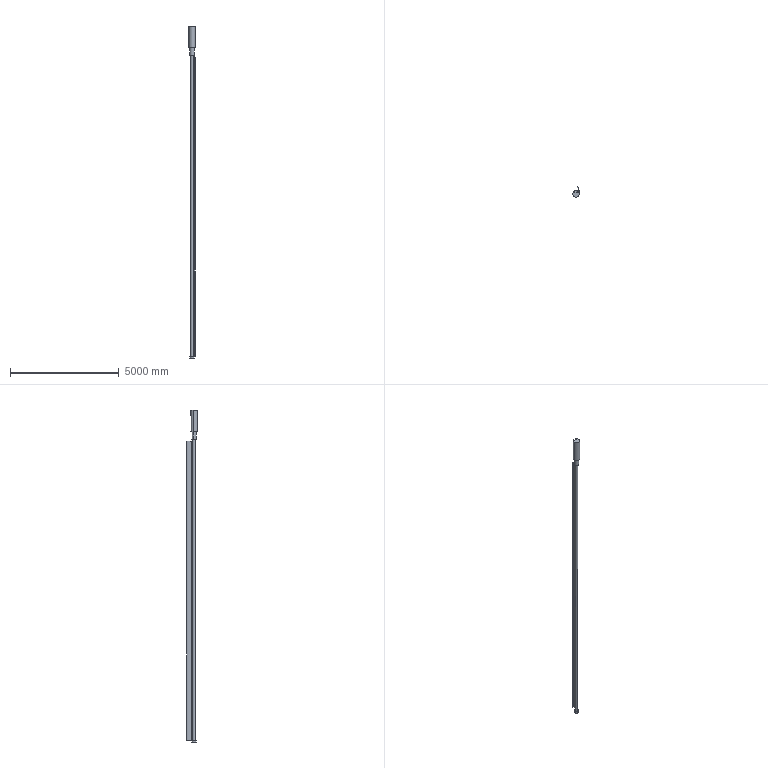Part | SolidWorks | features ICE 6, Extrusion 1 | 1 solid | 28 faces | box 300 x 474.612 x 15244 mm | volume 386924782 mm3 | plane 19 | cylinder 9 | commonest cylinder face diameters 200 x4 100 x2 300 x2 117.35 x1
STEP:
#1=CARTESIAN_POINT('',(50.,141.421,1160.));
#2=VERTEX_POINT('',#1);
#3=CARTESIAN_POINT('',(0.,150.,1110.));
#4=VERTEX_POINT('',#3);
#5=CARTESIAN_POINT('',(50.,141.421,1160.));
#6=CARTESIAN_POINT('',(50.,141.421,1156.669));
#7=CARTESIAN_POINT('',(49.671,141.539,1153.4));
#8=CARTESIAN_POINT('',(48.706,141.873,1148.582));
#9=CARTESIAN_POINT('',(48.306,142.01,1146.99));
#10=CARTESIAN_POINT('',(47.584,142.253,1144.624));
#11=CARTESIAN_POINT('',(47.323,142.34,1143.837));
#12=CARTESIAN_POINT('',(46.764,142.524,1142.286));
#13=CARTESIAN_POINT('',(46.467,142.622,1141.52));
#14=CARTESIAN_POINT('',(44.893,143.131,1137.743));
#15=CARTESIAN_POINT('',(43.355,143.61,1134.88));
#16=CARTESIAN_POINT('',(41.086,144.264,1131.494));
#17=CARTESIAN_POINT('',(40.615,144.398,1130.827));
#18=CARTESIAN_POINT('',(39.637,144.669,1129.511));
#19=CARTESIAN_POINT('',(39.132,144.807,1128.865));
#20=CARTESIAN_POINT('',(37.577,145.221,1126.975));
#21=CARTESIAN_POINT('',(36.486,145.5,1125.774));
#22=CARTESIAN_POINT('',(33.051,146.332,1122.342));
#23=CARTESIAN_POINT('',(30.547,146.883,1120.28));
#24=CARTESIAN_POINT('',(25.084,147.914,1116.623));
#25=CARTESIAN_POINT('',(22.213,148.377,1115.087));
#26=CARTESIAN_POINT('',(17.703,148.959,1113.211));
#27=CARTESIAN_POINT('',(16.166,149.135,1112.657));
#28=CARTESIAN_POINT('',(13.807,149.365,1111.937));
#29=CARTESIAN_POINT('',(13.012,149.437,1111.716));
#30=CARTESIAN_POINT('',(11.403,149.568,1111.311));
#31=CARTESIAN_POINT('',(10.595,149.628,1111.129));
#32=CARTESIAN_POINT('',(6.552,149.892,1110.322));
#33=CARTESIAN_POINT('',(3.29,150.,1110.));
#34=CARTESIAN_POINT('',(0.,150.,1110.));
#35=B_SPLINE_CURVE_WITH_KNOTS('',3,(#5,#6,#7,#8,#9,#10,#11,#12,#13,#14,#15,#16,#17,#18,#19,#20,#21,#22,#23,#24,#25,#26,#27,#28,#29,#30,#31,#32,#33,#34),.UNSPECIFIED.,.F.,.F.,(4,2,2,2,2,2,2,2,2,2,2,2,2,2,4),(0.,0.009844,0.01477,0.01723,0.01969,0.02953,0.03199,0.03445,0.03937,0.04922,0.05906,0.06398,0.06645,0.06891,0.07875),.UNSPECIFIED.);
#36=EDGE_CURVE('',#2,#4,#35,.T.);
#37=ORIENTED_EDGE('',*,*,#36,.T.);
#38=CARTESIAN_POINT('',(0.,75.,1110.));
#39=VERTEX_POINT('',#38);
#40=CARTESIAN_POINT('',(0.,326.,1110.));
#41=DIRECTION('',(0.,-1.,0.));
#42=VECTOR('',#41,1000.);
#43=LINE('',#40,#42);
#44=EDGE_CURVE('',#4,#39,#43,.T.);
#45=ORIENTED_EDGE('',*,*,#44,.T.);
#46=CARTESIAN_POINT('',(50.,75.,1160.));
#47=VERTEX_POINT('',#46);
#48=CARTESIAN_POINT('',(0.,75.,1160.));
#49=DIRECTION('',(0.,1.,0.));
#50=DIRECTION('',(0.,0.,1.));
#51=AXIS2_PLACEMENT_3D('',#48,#49,#50);
#52=CIRCLE('',#51,50.);
#53=EDGE_CURVE('',#47,#39,#52,.T.);
#54=ORIENTED_EDGE('',*,*,#53,.F.);
#55=CARTESIAN_POINT('',(50.,326.,1160.));
#56=DIRECTION('',(0.,-1.,0.));
#57=VECTOR('',#56,1000.);
#58=LINE('',#55,#57);
#59=EDGE_CURVE('',#2,#47,#58,.T.);
#60=ORIENTED_EDGE('',*,*,#59,.F.);
#61=EDGE_LOOP('',(#37,#45,#54,#60));
#62=FACE_OUTER_BOUND('',#61,.T.);
#63=CARTESIAN_POINT('',(0.,326.,1160.));
#64=DIRECTION('',(0.,-1.,0.));
#65=DIRECTION('',(0.,0.,-1.));
#66=AXIS2_PLACEMENT_3D('',#63,#64,#65);
#67=CYLINDRICAL_SURFACE('',#66,50.);
#68=ADVANCED_FACE('',(#62),#67,.F.);
#69=CARTESIAN_POINT('',(-100.,0.,-13904.));
#70=VERTEX_POINT('',#69);
#71=CARTESIAN_POINT('',(100.,0.,-13904.));
#72=VERTEX_POINT('',#71);
#73=CARTESIAN_POINT('',(0.,0.,-13904.));
#74=DIRECTION('',(0.,0.,-1.));
#75=DIRECTION('',(-1.,0.,0.));
#76=AXIS2_PLACEMENT_3D('',#73,#74,#75);
#77=CIRCLE('',#76,100.);
#78=EDGE_CURVE('',#70,#72,#77,.T.);
#79=ORIENTED_EDGE('',*,*,#78,.F.);
#80=CARTESIAN_POINT('',(-100.,0.,-13824.));
#81=VERTEX_POINT('',#80);
#82=CARTESIAN_POINT('',(-100.,0.,-13904.));
#83=DIRECTION('',(0.,0.,1.));
#84=VECTOR('',#83,1000.);
#85=LINE('',#82,#84);
#86=EDGE_CURVE('',#70,#81,#85,.T.);
#87=ORIENTED_EDGE('',*,*,#86,.T.);
#88=CARTESIAN_POINT('',(61.826,78.598,-13824.));
#89=VERTEX_POINT('',#88);
#90=CARTESIAN_POINT('',(0.,0.,-13824.));
#91=DIRECTION('',(0.,0.,-1.));
#92=DIRECTION('',(-1.,0.,0.));
#93=AXIS2_PLACEMENT_3D('',#90,#91,#92);
#94=CIRCLE('',#93,100.);
#95=EDGE_CURVE('',#81,#89,#94,.T.);
#96=ORIENTED_EDGE('',*,*,#95,.T.);
#97=CARTESIAN_POINT('',(96.233,27.187,-13824.));
#98=VERTEX_POINT('',#97);
#99=CARTESIAN_POINT('',(0.,0.,-13824.));
#100=DIRECTION('',(0.,0.,-1.));
#101=DIRECTION('',(-1.,0.,0.));
#102=AXIS2_PLACEMENT_3D('',#99,#100,#101);
#103=CIRCLE('',#102,100.);
#104=EDGE_CURVE('',#89,#98,#103,.T.);
#105=ORIENTED_EDGE('',*,*,#104,.T.);
#106=CARTESIAN_POINT('',(100.,0.,-13824.));
#107=VERTEX_POINT('',#106);
#108=CARTESIAN_POINT('',(0.,0.,-13824.));
#109=DIRECTION('',(0.,0.,-1.));
#110=DIRECTION('',(-1.,0.,0.));
#111=AXIS2_PLACEMENT_3D('',#108,#109,#110);
#112=CIRCLE('',#111,100.);
#113=EDGE_CURVE('',#98,#107,#112,.T.);
#114=ORIENTED_EDGE('',*,*,#113,.T.);
#115=CARTESIAN_POINT('',(100.,0.,-13904.));
#116=DIRECTION('',(0.,0.,1.));
#117=VECTOR('',#116,1000.);
#118=LINE('',#115,#117);
#119=EDGE_CURVE('',#72,#107,#118,.T.);
#120=ORIENTED_EDGE('',*,*,#119,.F.);
#121=EDGE_LOOP('',(#79,#87,#96,#105,#114,#120));
#122=FACE_OUTER_BOUND('',#121,.T.);
#123=CARTESIAN_POINT('',(0.,0.,-13904.));
#124=DIRECTION('',(0.,0.,1.));
#125=DIRECTION('',(1.,0.,0.));
#126=AXIS2_PLACEMENT_3D('',#123,#124,#125);
#127=CYLINDRICAL_SURFACE('',#126,100.);
#128=ADVANCED_FACE('',(#122),#127,.T.);
#129=CARTESIAN_POINT('',(100.,0.,340.));
#130=VERTEX_POINT('',#129);
#131=CARTESIAN_POINT('',(-100.,0.,340.));
#132=VERTEX_POINT('',#131);
#133=CARTESIAN_POINT('',(0.,0.,340.));
#134=DIRECTION('',(0.,0.,1.));
#135=DIRECTION('',(1.,0.,0.));
#136=AXIS2_PLACEMENT_3D('',#133,#134,#135);
#137=CIRCLE('',#136,100.);
#138=EDGE_CURVE('',#130,#132,#137,.T.);
#139=ORIENTED_EDGE('',*,*,#138,.F.);
#140=CARTESIAN_POINT('',(100.,0.,0.));
#141=VERTEX_POINT('',#140);
#142=CARTESIAN_POINT('',(100.,0.,340.));
#143=DIRECTION('',(0.,0.,-1.));
#144=VECTOR('',#143,1000.);
#145=LINE('',#142,#144);
#146=EDGE_CURVE('',#130,#141,#145,.T.);
#147=ORIENTED_EDGE('',*,*,#146,.T.);
#148=CARTESIAN_POINT('',(96.233,27.187,0.));
#149=VERTEX_POINT('',#148);
#150=CARTESIAN_POINT('',(0.,0.,0.));
#151=DIRECTION('',(0.,0.,1.));
#152=DIRECTION('',(1.,0.,0.));
#153=AXIS2_PLACEMENT_3D('',#150,#151,#152);
#154=CIRCLE('',#153,100.);
#155=EDGE_CURVE('',#141,#149,#154,.T.);
#156=ORIENTED_EDGE('',*,*,#155,.T.);
#157=CARTESIAN_POINT('',(96.233,27.187,-100.));
#158=VERTEX_POINT('',#157);
#159=CARTESIAN_POINT('',(96.233,27.187,-100.));
#160=DIRECTION('',(0.,0.,1.));
#161=VECTOR('',#160,1000.);
#162=LINE('',#159,#161);
#163=EDGE_CURVE('',#158,#149,#162,.T.);
#164=ORIENTED_EDGE('',*,*,#163,.F.);
#165=CARTESIAN_POINT('',(61.826,78.598,-100.));
#166=VERTEX_POINT('',#165);
#167=CARTESIAN_POINT('',(0.,0.,-100.));
#168=DIRECTION('',(0.,0.,-1.));
#169=DIRECTION('',(1.,0.,0.));
#170=AXIS2_PLACEMENT_3D('',#167,#168,#169);
#171=CIRCLE('',#170,100.);
#172=EDGE_CURVE('',#166,#158,#171,.T.);
#173=ORIENTED_EDGE('',*,*,#172,.F.);
#174=CARTESIAN_POINT('',(61.826,78.598,0.));
#175=VERTEX_POINT('',#174);
#176=CARTESIAN_POINT('',(61.826,78.598,-100.));
#177=DIRECTION('',(0.,0.,1.));
#178=VECTOR('',#177,1000.);
#179=LINE('',#176,#178);
#180=EDGE_CURVE('',#166,#175,#179,.T.);
#181=ORIENTED_EDGE('',*,*,#180,.T.);
#182=CARTESIAN_POINT('',(-100.,0.,0.));
#183=VERTEX_POINT('',#182);
#184=CARTESIAN_POINT('',(0.,0.,0.));
#185=DIRECTION('',(0.,0.,1.));
#186=DIRECTION('',(1.,0.,0.));
#187=AXIS2_PLACEMENT_3D('',#184,#185,#186);
#188=CIRCLE('',#187,100.);
#189=EDGE_CURVE('',#175,#183,#188,.T.);
#190=ORIENTED_EDGE('',*,*,#189,.T.);
#191=CARTESIAN_POINT('',(-100.,0.,340.));
#192=DIRECTION('',(0.,0.,-1.));
#193=VECTOR('',#192,1000.);
#194=LINE('',#191,#193);
#195=EDGE_CURVE('',#132,#183,#194,.T.);
#196=ORIENTED_EDGE('',*,*,#195,.F.);
#197=EDGE_LOOP('',(#139,#147,#156,#164,#173,#181,#190,#196));
#198=FACE_OUTER_BOUND('',#197,.T.);
#199=CARTESIAN_POINT('',(0.,0.,340.));
#200=DIRECTION('',(0.,0.,-1.));
#201=DIRECTION('',(-1.,0.,0.));
#202=AXIS2_PLACEMENT_3D('',#199,#200,#201);
#203=CYLINDRICAL_SURFACE('',#202,100.);
#204=ADVANCED_FACE('',(#198),#203,.T.);
#205=CARTESIAN_POINT('',(150.,0.,1340.));
#206=VERTEX_POINT('',#205);
#207=CARTESIAN_POINT('',(50.,141.421,1340.));
#208=VERTEX_POINT('',#207);
#209=CARTESIAN_POINT('',(0.,0.,1340.));
#210=DIRECTION('',(0.,0.,1.));
#211=DIRECTION('',(1.,0.,0.));
#212=AXIS2_PLACEMENT_3D('',#209,#210,#211);
#213=CIRCLE('',#212,150.);
#214=EDGE_CURVE('',#206,#208,#213,.T.);
#215=ORIENTED_EDGE('',*,*,#214,.F.);
#216=CARTESIAN_POINT('',(150.,0.,340.));
#217=VERTEX_POINT('',#216);
#218=CARTESIAN_POINT('',(150.,0.,1340.));
#219=DIRECTION('',(0.,0.,-1.));
#220=VECTOR('',#219,1000.);
#221=LINE('',#218,#220);
#222=EDGE_CURVE('',#206,#217,#221,.T.);
#223=ORIENTED_EDGE('',*,*,#222,.T.);
#224=CARTESIAN_POINT('',(-150.,0.,340.));
#225=VERTEX_POINT('',#224);
#226=CARTESIAN_POINT('',(0.,0.,340.));
#227=DIRECTION('',(0.,0.,1.));
#228=DIRECTION('',(1.,0.,0.));
#229=AXIS2_PLACEMENT_3D('',#226,#227,#228);
#230=CIRCLE('',#229,150.);
#231=EDGE_CURVE('',#217,#225,#230,.T.);
#232=ORIENTED_EDGE('',*,*,#231,.T.);
#233=CARTESIAN_POINT('',(-150.,0.,1340.));
#234=VERTEX_POINT('',#233);
#235=CARTESIAN_POINT('',(-150.,0.,1340.));
#236=DIRECTION('',(0.,0.,-1.));
#237=VECTOR('',#236,1000.);
#238=LINE('',#235,#237);
#239=EDGE_CURVE('',#234,#225,#238,.T.);
#240=ORIENTED_EDGE('',*,*,#239,.F.);
#241=CARTESIAN_POINT('',(-50.,141.421,1340.));
#242=VERTEX_POINT('',#241);
#243=CARTESIAN_POINT('',(0.,0.,1340.));
#244=DIRECTION('',(0.,0.,1.));
#245=DIRECTION('',(1.,0.,0.));
#246=AXIS2_PLACEMENT_3D('',#243,#244,#245);
#247=CIRCLE('',#246,150.);
#248=EDGE_CURVE('',#242,#234,#247,.T.);
#249=ORIENTED_EDGE('',*,*,#248,.F.);
#250=CARTESIAN_POINT('',(-50.,141.421,1160.));
#251=VERTEX_POINT('',#250);
#252=CARTESIAN_POINT('',(-50.,141.421,1340.));
#253=DIRECTION('',(0.,0.,1.));
#254=VECTOR('',#253,1000.);
#255=LINE('',#252,#254);
#256=EDGE_CURVE('',#251,#242,#255,.T.);
#257=ORIENTED_EDGE('',*,*,#256,.F.);
#258=CARTESIAN_POINT('',(0.,150.,1110.));
#259=CARTESIAN_POINT('',(-0.8214,150.,1110.));
#260=CARTESIAN_POINT('',(-1.644,149.993,1110.02));
#261=CARTESIAN_POINT('',(-3.294,149.966,1110.102));
#262=CARTESIAN_POINT('',(-4.123,149.946,1110.163));
#263=CARTESIAN_POINT('',(-6.6,149.864,1110.41));
#264=CARTESIAN_POINT('',(-8.228,149.783,1110.654));
#265=CARTESIAN_POINT('',(-13.049,149.466,1111.622));
#266=CARTESIAN_POINT('',(-16.176,149.157,1112.574));
#267=CARTESIAN_POINT('',(-19.976,148.666,1114.156));
#268=CARTESIAN_POINT('',(-20.73,148.563,1114.492));
#269=CARTESIAN_POINT('',(-22.211,148.348,1115.197));
#270=CARTESIAN_POINT('',(-22.94,148.237,1115.566));
#271=CARTESIAN_POINT('',(-25.094,147.893,1116.722));
#272=CARTESIAN_POINT('',(-26.484,147.65,1117.559));
#273=CARTESIAN_POINT('',(-29.178,147.141,1119.364));
#274=CARTESIAN_POINT('',(-30.481,146.876,1120.332));
#275=CARTESIAN_POINT('',(-32.369,146.467,1121.883));
#276=CARTESIAN_POINT('',(-32.988,146.329,1122.417));
#277=CARTESIAN_POINT('',(-34.2,146.05,1123.517));
#278=CARTESIAN_POINT('',(-34.791,145.911,1124.08));
#279=CARTESIAN_POINT('',(-37.664,145.214,1126.955));
#280=CARTESIAN_POINT('',(-39.715,144.659,1129.451));
#281=CARTESIAN_POINT('',(-41.976,144.008,1132.821));
#282=CARTESIAN_POINT('',(-42.413,143.88,1133.508));
#283=CARTESIAN_POINT('',(-43.255,143.629,1134.907));
#284=CARTESIAN_POINT('',(-43.662,143.505,1135.621));
#285=CARTESIAN_POINT('',(-44.827,143.147,1137.791));
#286=CARTESIAN_POINT('',(-45.528,142.925,1139.266));
#287=CARTESIAN_POINT('',(-47.406,142.318,1143.774));
#288=CARTESIAN_POINT('',(-48.363,141.991,1146.889));
#289=CARTESIAN_POINT('',(-49.177,141.71,1150.928));
#290=CARTESIAN_POINT('',(-49.321,141.66,1151.745));
#291=CARTESIAN_POINT('',(-49.568,141.574,1153.386));
#292=CARTESIAN_POINT('',(-49.67,141.538,1154.208));
#293=CARTESIAN_POINT('',(-49.917,141.451,1156.681));
#294=CARTESIAN_POINT('',(-50.,141.421,1158.337));
#295=CARTESIAN_POINT('',(-50.,141.421,1160.));
#296=B_SPLINE_CURVE_WITH_KNOTS('',3,(#258,#259,#260,#261,#262,#263,#264,#265,#266,#267,#268,#269,#270,#271,#272,#273,#274,#275,#276,#277,#278,#279,#280,#281,#282,#283,#284,#285,#286,#287,#288,#289,#290,#291,#292,#293,#294,#295),.UNSPECIFIED.,.F.,.F.,(4,2,2,2,2,2,2,2,2,2,2,2,2,2,2,2,2,2,4),(0.07875,0.08121,0.08366,0.08858,0.09841,0.1009,0.1033,0.1082,0.1132,0.1156,0.1181,0.1279,0.1304,0.1328,0.1377,0.1476,0.15,0.1525,0.1574),.UNSPECIFIED.);
#297=EDGE_CURVE('',#4,#251,#296,.T.);
#298=ORIENTED_EDGE('',*,*,#297,.F.);
#299=ORIENTED_EDGE('',*,*,#36,.F.);
#300=CARTESIAN_POINT('',(50.,141.421,1340.));
#301=DIRECTION('',(0.,0.,-1.));
#302=VECTOR('',#301,1000.);
#303=LINE('',#300,#302);
#304=EDGE_CURVE('',#208,#2,#303,.T.);
#305=ORIENTED_EDGE('',*,*,#304,.F.);
#306=EDGE_LOOP('',(#215,#223,#232,#240,#249,#257,#298,#299,#305));
#307=FACE_OUTER_BOUND('',#306,.T.);
#308=CARTESIAN_POINT('',(0.,0.,1340.));
#309=DIRECTION('',(0.,0.,-1.));
#310=DIRECTION('',(-1.,0.,0.));
#311=AXIS2_PLACEMENT_3D('',#308,#309,#310);
#312=CYLINDRICAL_SURFACE('',#311,150.);
#313=ADVANCED_FACE('',(#307),#312,.T.);
#314=ORIENTED_EDGE('',*,*,#222,.F.);
#315=CARTESIAN_POINT('',(0.,0.,1340.));
#316=DIRECTION('',(0.,0.,1.));
#317=DIRECTION('',(1.,0.,0.));
#318=AXIS2_PLACEMENT_3D('',#315,#316,#317);
#319=CIRCLE('',#318,150.);
#320=EDGE_CURVE('',#234,#206,#319,.T.);
#321=ORIENTED_EDGE('',*,*,#320,.F.);
#322=ORIENTED_EDGE('',*,*,#239,.T.);
#323=CARTESIAN_POINT('',(0.,0.,340.));
#324=DIRECTION('',(0.,0.,1.));
#325=DIRECTION('',(1.,0.,0.));
#326=AXIS2_PLACEMENT_3D('',#323,#324,#325);
#327=CIRCLE('',#326,150.);
#328=EDGE_CURVE('',#225,#217,#327,.T.);
#329=ORIENTED_EDGE('',*,*,#328,.T.);
#330=EDGE_LOOP('',(#314,#321,#322,#329));
#331=FACE_OUTER_BOUND('',#330,.T.);
#332=CARTESIAN_POINT('',(0.,0.,1340.));
#333=DIRECTION('',(0.,0.,-1.));
#334=DIRECTION('',(-1.,0.,0.));
#335=AXIS2_PLACEMENT_3D('',#332,#333,#334);
#336=CYLINDRICAL_SURFACE('',#335,150.);
#337=ADVANCED_FACE('',(#331),#336,.T.);
#338=CARTESIAN_POINT('',(-50.,75.,1340.));
#339=VERTEX_POINT('',#338);
#340=CARTESIAN_POINT('',(50.,75.,1340.));
#341=VERTEX_POINT('',#340);
#342=CARTESIAN_POINT('',(-50.,75.,1340.));
#343=DIRECTION('',(1.,0.,0.));
#344=VECTOR('',#343,1000.);
#345=LINE('',#342,#344);
#346=EDGE_CURVE('',#339,#341,#345,.T.);
#347=ORIENTED_EDGE('',*,*,#346,.F.);
#348=CARTESIAN_POINT('',(-50.,0.,1340.));
#349=DIRECTION('',(0.,1.,0.));
#350=VECTOR('',#349,1000.);
#351=LINE('',#348,#350);
#352=EDGE_CURVE('',#339,#242,#351,.T.);
#353=ORIENTED_EDGE('',*,*,#352,.T.);
#354=ORIENTED_EDGE('',*,*,#248,.T.);
#355=ORIENTED_EDGE('',*,*,#320,.T.);
#356=ORIENTED_EDGE('',*,*,#214,.T.);
#357=CARTESIAN_POINT('',(50.,0.,1340.));
#358=DIRECTION('',(0.,-1.,0.));
#359=VECTOR('',#358,1000.);
#360=LINE('',#357,#359);
#361=EDGE_CURVE('',#208,#341,#360,.T.);
#362=ORIENTED_EDGE('',*,*,#361,.T.);
#363=EDGE_LOOP('',(#347,#353,#354,#355,#356,#362));
#364=FACE_OUTER_BOUND('',#363,.T.);
#365=CARTESIAN_POINT('',(0.,0.,1340.));
#366=DIRECTION('',(0.,0.,1.));
#367=DIRECTION('',(1.,0.,0.));
#368=AXIS2_PLACEMENT_3D('',#365,#366,#367);
#369=PLANE('',#368);
#370=ADVANCED_FACE('',(#364),#369,.T.);
#371=CARTESIAN_POINT('',(127.239,110.96,-100.));
#372=VERTEX_POINT('',#371);
#373=CARTESIAN_POINT('',(127.239,110.96,-100.));
#374=DIRECTION('',(-0.8963,-0.4434,0.));
#375=VECTOR('',#374,1000.);
#376=LINE('',#373,#375);
#377=EDGE_CURVE('',#372,#166,#376,.T.);
#378=ORIENTED_EDGE('',*,*,#377,.F.);
#379=CARTESIAN_POINT('',(127.239,110.96,-13824.));
#380=VERTEX_POINT('',#379);
#381=CARTESIAN_POINT('',(127.239,110.96,-13824.));
#382=DIRECTION('',(0.,0.,1.));
#383=VECTOR('',#382,1000.);
#384=LINE('',#381,#383);
#385=EDGE_CURVE('',#380,#372,#384,.T.);
#386=ORIENTED_EDGE('',*,*,#385,.F.);
#387=CARTESIAN_POINT('',(127.239,110.96,-13824.));
#388=DIRECTION('',(0.8963,0.4434,0.));
#389=VECTOR('',#388,1000.);
#390=LINE('',#387,#389);
#391=EDGE_CURVE('',#89,#380,#390,.T.);
#392=ORIENTED_EDGE('',*,*,#391,.F.);
#393=CARTESIAN_POINT('',(61.826,78.598,-13824.));
#394=DIRECTION('',(0.,0.,1.));
#395=VECTOR('',#394,1000.);
#396=LINE('',#393,#395);
#397=EDGE_CURVE('',#89,#166,#396,.T.);
#398=ORIENTED_EDGE('',*,*,#397,.T.);
#399=EDGE_LOOP('',(#378,#386,#392,#398));
#400=FACE_OUTER_BOUND('',#399,.T.);
#401=CARTESIAN_POINT('',(127.239,110.96,-13824.));
#402=DIRECTION('',(0.4434,-0.8963,0.));
#403=DIRECTION('',(0.8963,0.4434,0.));
#404=AXIS2_PLACEMENT_3D('',#401,#402,#403);
#405=PLANE('',#404);
#406=ADVANCED_FACE('',(#400),#405,.F.);
#407=CARTESIAN_POINT('',(106.547,286.808,-100.));
#408=VERTEX_POINT('',#407);
#409=CARTESIAN_POINT('',(106.547,286.808,-100.));
#410=DIRECTION('',(0.1169,-0.9931,0.));
#411=VECTOR('',#410,1000.);
#412=LINE('',#409,#411);
#413=EDGE_CURVE('',#408,#372,#412,.T.);
#414=ORIENTED_EDGE('',*,*,#413,.F.);
#415=CARTESIAN_POINT('',(106.547,286.808,-13824.));
#416=VERTEX_POINT('',#415);
#417=CARTESIAN_POINT('',(106.547,286.808,-13824.));
#418=DIRECTION('',(0.,0.,1.));
#419=VECTOR('',#418,1000.);
#420=LINE('',#417,#419);
#421=EDGE_CURVE('',#416,#408,#420,.T.);
#422=ORIENTED_EDGE('',*,*,#421,.F.);
#423=CARTESIAN_POINT('',(106.547,286.808,-13824.));
#424=DIRECTION('',(-0.1169,0.9931,0.));
#425=VECTOR('',#424,1000.);
#426=LINE('',#423,#425);
#427=EDGE_CURVE('',#380,#416,#426,.T.);
#428=ORIENTED_EDGE('',*,*,#427,.F.);
#429=ORIENTED_EDGE('',*,*,#385,.T.);
#430=EDGE_LOOP('',(#414,#422,#428,#429));
#431=FACE_OUTER_BOUND('',#430,.T.);
#432=CARTESIAN_POINT('',(106.547,286.808,-13824.));
#433=DIRECTION('',(0.9931,0.1169,0.));
#434=DIRECTION('',(-0.1169,0.9931,0.));
#435=AXIS2_PLACEMENT_3D('',#432,#433,#434);
#436=PLANE('',#435);
#437=ADVANCED_FACE('',(#431),#436,.F.);
#438=CARTESIAN_POINT('',(53.816,324.612,-100.));
#439=VERTEX_POINT('',#438);
#440=CARTESIAN_POINT('',(53.816,324.612,-100.));
#441=DIRECTION('',(0.8127,-0.5827,0.));
#442=VECTOR('',#441,1000.);
#443=LINE('',#440,#442);
#444=EDGE_CURVE('',#439,#408,#443,.T.);
#445=ORIENTED_EDGE('',*,*,#444,.F.);
#446=CARTESIAN_POINT('',(53.816,324.612,-13824.));
#447=VERTEX_POINT('',#446);
#448=CARTESIAN_POINT('',(53.816,324.612,-13824.));
#449=DIRECTION('',(0.,0.,1.));
#450=VECTOR('',#449,1000.);
#451=LINE('',#448,#450);
#452=EDGE_CURVE('',#447,#439,#451,.T.);
#453=ORIENTED_EDGE('',*,*,#452,.F.);
#454=CARTESIAN_POINT('',(69.836,313.127,-13824.));
#455=DIRECTION('',(-0.8127,0.5827,0.));
#456=VECTOR('',#455,1000.);
#457=LINE('',#454,#456);
#458=EDGE_CURVE('',#416,#447,#457,.T.);
#459=ORIENTED_EDGE('',*,*,#458,.F.);
#460=ORIENTED_EDGE('',*,*,#421,.T.);
#461=EDGE_LOOP('',(#445,#453,#459,#460));
#462=FACE_OUTER_BOUND('',#461,.T.);
#463=CARTESIAN_POINT('',(53.816,324.612,-13824.));
#464=DIRECTION('',(0.5827,0.8127,0.));
#465=DIRECTION('',(-0.8127,0.5827,0.));
#466=AXIS2_PLACEMENT_3D('',#463,#464,#465);
#467=PLANE('',#466);
#468=ADVANCED_FACE('',(#462),#467,.F.);
#469=CARTESIAN_POINT('',(85.855,324.612,-100.));
#470=VERTEX_POINT('',#469);
#471=CARTESIAN_POINT('',(85.855,324.612,-100.));
#472=DIRECTION('',(-1.,0.,0.));
#473=VECTOR('',#472,1000.);
#474=LINE('',#471,#473);
#475=EDGE_CURVE('',#470,#439,#474,.T.);
#476=ORIENTED_EDGE('',*,*,#475,.F.);
#477=CARTESIAN_POINT('',(85.855,324.612,-13824.));
#478=VERTEX_POINT('',#477);
#479=CARTESIAN_POINT('',(85.855,324.612,-13824.));
#480=DIRECTION('',(0.,0.,1.));
#481=VECTOR('',#480,1000.);
#482=LINE('',#479,#481);
#483=EDGE_CURVE('',#478,#470,#482,.T.);
#484=ORIENTED_EDGE('',*,*,#483,.F.);
#485=CARTESIAN_POINT('',(85.855,324.612,-13824.));
#486=DIRECTION('',(1.,0.,0.));
#487=VECTOR('',#486,1000.);
#488=LINE('',#485,#487);
#489=EDGE_CURVE('',#447,#478,#488,.T.);
#490=ORIENTED_EDGE('',*,*,#489,.F.);
#491=ORIENTED_EDGE('',*,*,#452,.T.);
#492=EDGE_LOOP('',(#476,#484,#490,#491));
#493=FACE_OUTER_BOUND('',#492,.T.);
#494=CARTESIAN_POINT('',(85.855,324.612,-13824.));
#495=DIRECTION('',(0.,-1.,0.));
#496=DIRECTION('',(0.,0.,-1.));
#497=AXIS2_PLACEMENT_3D('',#494,#495,#496);
#498=PLANE('',#497);
#499=ADVANCED_FACE('',(#493),#498,.F.);
#500=CARTESIAN_POINT('',(127.239,294.943,-100.));
#501=VERTEX_POINT('',#500);
#502=CARTESIAN_POINT('',(127.239,294.943,-100.));
#503=DIRECTION('',(-0.8127,0.5827,0.));
#504=VECTOR('',#503,1000.);
#505=LINE('',#502,#504);
#506=EDGE_CURVE('',#501,#470,#505,.T.);
#507=ORIENTED_EDGE('',*,*,#506,.F.);
#508=CARTESIAN_POINT('',(127.239,294.943,-13824.));
#509=VERTEX_POINT('',#508);
#510=CARTESIAN_POINT('',(127.239,294.943,-13824.));
#511=DIRECTION('',(0.,0.,1.));
#512=VECTOR('',#511,1000.);
#513=LINE('',#510,#512);
#514=EDGE_CURVE('',#509,#501,#513,.T.);
#515=ORIENTED_EDGE('',*,*,#514,.F.);
#516=CARTESIAN_POINT('',(127.239,294.943,-13824.));
#517=DIRECTION('',(0.8127,-0.5827,0.));
#518=VECTOR('',#517,1000.);
#519=LINE('',#516,#518);
#520=EDGE_CURVE('',#478,#509,#519,.T.);
#521=ORIENTED_EDGE('',*,*,#520,.F.);
#522=ORIENTED_EDGE('',*,*,#483,.T.);
#523=EDGE_LOOP('',(#507,#515,#521,#522));
#524=FACE_OUTER_BOUND('',#523,.T.);
#525=CARTESIAN_POINT('',(127.239,294.943,-13824.));
#526=DIRECTION('',(-0.5827,-0.8127,0.));
#527=DIRECTION('',(0.8127,-0.5827,0.));
#528=AXIS2_PLACEMENT_3D('',#525,#526,#527);
#529=PLANE('',#528);
#530=ADVANCED_FACE('',(#524),#529,.F.);
#531=CARTESIAN_POINT('',(146.429,97.202,-100.));
#532=VERTEX_POINT('',#531);
#533=CARTESIAN_POINT('',(146.429,97.202,-100.));
#534=DIRECTION('',(-0.09659,0.9953,0.));
#535=VECTOR('',#534,1000.);
#536=LINE('',#533,#535);
#537=EDGE_CURVE('',#532,#501,#536,.T.);
#538=ORIENTED_EDGE('',*,*,#537,.F.);
#539=CARTESIAN_POINT('',(146.429,97.202,-13824.));
#540=VERTEX_POINT('',#539);
#541=CARTESIAN_POINT('',(146.429,97.202,-13824.));
#542=DIRECTION('',(0.,0.,1.));
#543=VECTOR('',#542,1000.);
#544=LINE('',#541,#543);
#545=EDGE_CURVE('',#540,#532,#544,.T.);
#546=ORIENTED_EDGE('',*,*,#545,.F.);
#547=CARTESIAN_POINT('',(146.429,97.202,-13824.));
#548=DIRECTION('',(0.09659,-0.9953,0.));
#549=VECTOR('',#548,1000.);
#550=LINE('',#547,#549);
#551=EDGE_CURVE('',#509,#540,#550,.T.);
#552=ORIENTED_EDGE('',*,*,#551,.F.);
#553=ORIENTED_EDGE('',*,*,#514,.T.);
#554=EDGE_LOOP('',(#538,#546,#552,#553));
#555=FACE_OUTER_BOUND('',#554,.T.);
#556=CARTESIAN_POINT('',(146.429,97.202,-13824.));
#557=DIRECTION('',(-0.9953,-0.09659,0.));
#558=DIRECTION('',(0.09659,-0.9953,0.));
#559=AXIS2_PLACEMENT_3D('',#556,#557,#558);
#560=PLANE('',#559);
#561=ADVANCED_FACE('',(#555),#560,.F.);
#562=CARTESIAN_POINT('',(96.233,27.187,-100.));
#563=DIRECTION('',(0.5827,0.8127,0.));
#564=VECTOR('',#563,1000.);
#565=LINE('',#562,#564);
#566=EDGE_CURVE('',#158,#532,#565,.T.);
#567=ORIENTED_EDGE('',*,*,#566,.F.);
#568=CARTESIAN_POINT('',(96.233,27.187,-13824.));
#569=DIRECTION('',(0.,0.,1.));
#570=VECTOR('',#569,1000.);
#571=LINE('',#568,#570);
#572=EDGE_CURVE('',#98,#158,#571,.T.);
#573=ORIENTED_EDGE('',*,*,#572,.F.);
#574=CARTESIAN_POINT('',(96.233,27.187,-13824.));
#575=DIRECTION('',(-0.5827,-0.8127,0.));
#576=VECTOR('',#575,1000.);
#577=LINE('',#574,#576);
#578=EDGE_CURVE('',#540,#98,#577,.T.);
#579=ORIENTED_EDGE('',*,*,#578,.F.);
#580=ORIENTED_EDGE('',*,*,#545,.T.);
#581=EDGE_LOOP('',(#567,#573,#579,#580));
#582=FACE_OUTER_BOUND('',#581,.T.);
#583=CARTESIAN_POINT('',(96.233,27.187,-13824.));
#584=DIRECTION('',(-0.8127,0.5827,0.));
#585=DIRECTION('',(-0.5827,-0.8127,0.));
#586=AXIS2_PLACEMENT_3D('',#583,#584,#585);
#587=PLANE('',#586);
#588=ADVANCED_FACE('',(#582),#587,.F.);
#589=ORIENTED_EDGE('',*,*,#146,.F.);
#590=CARTESIAN_POINT('',(0.,0.,340.));
#591=DIRECTION('',(0.,0.,1.));
#592=DIRECTION('',(1.,0.,0.));
#593=AXIS2_PLACEMENT_3D('',#590,#591,#592);
#594=CIRCLE('',#593,100.);
#595=EDGE_CURVE('',#132,#130,#594,.T.);
#596=ORIENTED_EDGE('',*,*,#595,.F.);
#597=ORIENTED_EDGE('',*,*,#195,.T.);
#598=CARTESIAN_POINT('',(0.,0.,0.));
#599=DIRECTION('',(0.,0.,1.));
#600=DIRECTION('',(1.,0.,0.));
#601=AXIS2_PLACEMENT_3D('',#598,#599,#600);
#602=CIRCLE('',#601,100.);
#603=EDGE_CURVE('',#183,#141,#602,.T.);
#604=ORIENTED_EDGE('',*,*,#603,.T.);
#605=EDGE_LOOP('',(#589,#596,#597,#604));
#606=FACE_OUTER_BOUND('',#605,.T.);
#607=CARTESIAN_POINT('',(0.,0.,340.));
#608=DIRECTION('',(0.,0.,-1.));
#609=DIRECTION('',(-1.,0.,0.));
#610=AXIS2_PLACEMENT_3D('',#607,#608,#609);
#611=CYLINDRICAL_SURFACE('',#610,100.);
#612=ADVANCED_FACE('',(#606),#611,.T.);
#613=CARTESIAN_POINT('',(48.187,-33.477,0.));
#614=VERTEX_POINT('',#613);
#615=CARTESIAN_POINT('',(96.233,27.187,0.));
#616=DIRECTION('',(-0.6209,-0.7839,0.));
#617=VECTOR('',#616,1000.);
#618=LINE('',#615,#617);
#619=EDGE_CURVE('',#149,#614,#618,.T.);
#620=ORIENTED_EDGE('',*,*,#619,.F.);
#621=ORIENTED_EDGE('',*,*,#155,.F.);
#622=ORIENTED_EDGE('',*,*,#603,.F.);
#623=ORIENTED_EDGE('',*,*,#189,.F.);
#624=CARTESIAN_POINT('',(0.,58.675,0.));
#625=VERTEX_POINT('',#624);
#626=CARTESIAN_POINT('',(61.826,78.598,0.));
#627=DIRECTION('',(0.9518,0.3067,0.));
#628=VECTOR('',#627,1000.);
#629=LINE('',#626,#628);
#630=EDGE_CURVE('',#625,#175,#629,.T.);
#631=ORIENTED_EDGE('',*,*,#630,.F.);
#632=CARTESIAN_POINT('',(0.,0.,0.));
#633=DIRECTION('',(0.,0.,-1.));
#634=DIRECTION('',(-1.,0.,0.));
#635=AXIS2_PLACEMENT_3D('',#632,#633,#634);
#636=CIRCLE('',#635,58.675);
#637=EDGE_CURVE('',#614,#625,#636,.T.);
#638=ORIENTED_EDGE('',*,*,#637,.F.);
#639=EDGE_LOOP('',(#620,#621,#622,#623,#631,#638));
#640=FACE_OUTER_BOUND('',#639,.T.);
#641=CARTESIAN_POINT('',(0.,0.,0.));
#642=DIRECTION('',(0.,0.,1.));
#643=DIRECTION('',(1.,0.,0.));
#644=AXIS2_PLACEMENT_3D('',#641,#642,#643);
#645=PLANE('',#644);
#646=ADVANCED_FACE('',(#640),#645,.F.);
#647=ORIENTED_EDGE('',*,*,#619,.T.);
#648=CARTESIAN_POINT('',(48.187,-33.477,-13824.));
#649=VERTEX_POINT('',#648);
#650=CARTESIAN_POINT('',(48.187,-33.477,-13824.));
#651=DIRECTION('',(0.,0.,1.));
#652=VECTOR('',#651,1000.);
#653=LINE('',#650,#652);
#654=EDGE_CURVE('',#649,#614,#653,.T.);
#655=ORIENTED_EDGE('',*,*,#654,.F.);
#656=CARTESIAN_POINT('',(96.233,27.187,-13824.));
#657=DIRECTION('',(-0.6209,-0.7839,0.));
#658=VECTOR('',#657,1000.);
#659=LINE('',#656,#658);
#660=EDGE_CURVE('',#98,#649,#659,.T.);
#661=ORIENTED_EDGE('',*,*,#660,.F.);
#662=ORIENTED_EDGE('',*,*,#572,.T.);
#663=ORIENTED_EDGE('',*,*,#163,.T.);
#664=EDGE_LOOP('',(#647,#655,#661,#662,#663));
#665=FACE_OUTER_BOUND('',#664,.T.);
#666=CARTESIAN_POINT('',(96.233,27.187,-13824.));
#667=DIRECTION('',(-0.7839,0.6209,0.));
#668=DIRECTION('',(-0.6209,-0.7839,0.));
#669=AXIS2_PLACEMENT_3D('',#666,#667,#668);
#670=PLANE('',#669);
#671=ADVANCED_FACE('',(#665),#670,.F.);
#672=ORIENTED_EDGE('',*,*,#637,.T.);
#673=CARTESIAN_POINT('',(0.,58.675,-13824.));
#674=VERTEX_POINT('',#673);
#675=CARTESIAN_POINT('',(0.,58.675,-13824.));
#676=DIRECTION('',(0.,0.,1.));
#677=VECTOR('',#676,1000.);
#678=LINE('',#675,#677);
#679=EDGE_CURVE('',#674,#625,#678,.T.);
#680=ORIENTED_EDGE('',*,*,#679,.F.);
#681=CARTESIAN_POINT('',(0.,0.,-13824.));
#682=DIRECTION('',(0.,0.,-1.));
#683=DIRECTION('',(-1.,0.,0.));
#684=AXIS2_PLACEMENT_3D('',#681,#682,#683);
#685=CIRCLE('',#684,58.675);
#686=EDGE_CURVE('',#649,#674,#685,.T.);
#687=ORIENTED_EDGE('',*,*,#686,.F.);
#688=ORIENTED_EDGE('',*,*,#654,.T.);
#689=EDGE_LOOP('',(#672,#680,#687,#688));
#690=FACE_OUTER_BOUND('',#689,.T.);
#691=CARTESIAN_POINT('',(0.,0.,-13824.));
#692=DIRECTION('',(0.,0.,1.));
#693=DIRECTION('',(1.,0.,0.));
#694=AXIS2_PLACEMENT_3D('',#691,#692,#693);
#695=CYLINDRICAL_SURFACE('',#694,58.675);
#696=ADVANCED_FACE('',(#690),#695,.T.);
#697=ORIENTED_EDGE('',*,*,#630,.T.);
#698=ORIENTED_EDGE('',*,*,#180,.F.);
#699=ORIENTED_EDGE('',*,*,#397,.F.);
#700=CARTESIAN_POINT('',(61.826,78.598,-13824.));
#701=DIRECTION('',(0.9518,0.3067,0.));
#702=VECTOR('',#701,1000.);
#703=LINE('',#700,#702);
#704=EDGE_CURVE('',#674,#89,#703,.T.);
#705=ORIENTED_EDGE('',*,*,#704,.F.);
#706=ORIENTED_EDGE('',*,*,#679,.T.);
#707=EDGE_LOOP('',(#697,#698,#699,#705,#706));
#708=FACE_OUTER_BOUND('',#707,.T.);
#709=CARTESIAN_POINT('',(61.826,78.598,-13824.));
#710=DIRECTION('',(0.3067,-0.9518,0.));
#711=DIRECTION('',(0.9518,0.3067,0.));
#712=AXIS2_PLACEMENT_3D('',#709,#710,#711);
#713=PLANE('',#712);
#714=ADVANCED_FACE('',(#708),#713,.F.);
#715=ORIENTED_EDGE('',*,*,#104,.F.);
#716=ORIENTED_EDGE('',*,*,#391,.T.);
#717=ORIENTED_EDGE('',*,*,#427,.T.);
#718=ORIENTED_EDGE('',*,*,#458,.T.);
#719=ORIENTED_EDGE('',*,*,#489,.T.);
#720=ORIENTED_EDGE('',*,*,#520,.T.);
#721=ORIENTED_EDGE('',*,*,#551,.T.);
#722=ORIENTED_EDGE('',*,*,#578,.T.);
#723=EDGE_LOOP('',(#715,#716,#717,#718,#719,#720,#721,#722));
#724=FACE_OUTER_BOUND('',#723,.T.);
#725=CARTESIAN_POINT('',(0.,0.,-13824.));
#726=DIRECTION('',(0.,0.,-1.));
#727=DIRECTION('',(-1.,0.,0.));
#728=AXIS2_PLACEMENT_3D('',#725,#726,#727);
#729=PLANE('',#728);
#730=ADVANCED_FACE('',(#724),#729,.T.);
#731=ORIENTED_EDGE('',*,*,#113,.F.);
#732=ORIENTED_EDGE('',*,*,#660,.T.);
#733=ORIENTED_EDGE('',*,*,#686,.T.);
#734=ORIENTED_EDGE('',*,*,#704,.T.);
#735=ORIENTED_EDGE('',*,*,#95,.F.);
#736=CARTESIAN_POINT('',(0.,0.,-13824.));
#737=DIRECTION('',(0.,0.,-1.));
#738=DIRECTION('',(-1.,0.,0.));
#739=AXIS2_PLACEMENT_3D('',#736,#737,#738);
#740=CIRCLE('',#739,100.);
#741=EDGE_CURVE('',#107,#81,#740,.T.);
#742=ORIENTED_EDGE('',*,*,#741,.F.);
#743=EDGE_LOOP('',(#731,#732,#733,#734,#735,#742));
#744=FACE_OUTER_BOUND('',#743,.T.);
#745=CARTESIAN_POINT('',(0.,0.,-13824.));
#746=DIRECTION('',(0.,0.,-1.));
#747=DIRECTION('',(-1.,0.,0.));
#748=AXIS2_PLACEMENT_3D('',#745,#746,#747);
#749=PLANE('',#748);
#750=ADVANCED_FACE('',(#744),#749,.F.);
#751=ORIENTED_EDGE('',*,*,#86,.F.);
#752=CARTESIAN_POINT('',(0.,0.,-13904.));
#753=DIRECTION('',(0.,0.,-1.));
#754=DIRECTION('',(-1.,0.,0.));
#755=AXIS2_PLACEMENT_3D('',#752,#753,#754);
#756=CIRCLE('',#755,100.);
#757=EDGE_CURVE('',#72,#70,#756,.T.);
#758=ORIENTED_EDGE('',*,*,#757,.F.);
#759=ORIENTED_EDGE('',*,*,#119,.T.);
#760=ORIENTED_EDGE('',*,*,#741,.T.);
#761=EDGE_LOOP('',(#751,#758,#759,#760));
#762=FACE_OUTER_BOUND('',#761,.T.);
#763=CARTESIAN_POINT('',(0.,0.,-13904.));
#764=DIRECTION('',(0.,0.,1.));
#765=DIRECTION('',(1.,0.,0.));
#766=AXIS2_PLACEMENT_3D('',#763,#764,#765);
#767=CYLINDRICAL_SURFACE('',#766,100.);
#768=ADVANCED_FACE('',(#762),#767,.T.);
#769=ORIENTED_EDGE('',*,*,#757,.T.);
#770=ORIENTED_EDGE('',*,*,#78,.T.);
#771=EDGE_LOOP('',(#769,#770));
#772=FACE_OUTER_BOUND('',#771,.T.);
#773=CARTESIAN_POINT('',(0.,0.,-13904.));
#774=DIRECTION('',(0.,0.,-1.));
#775=DIRECTION('',(-1.,0.,0.));
#776=AXIS2_PLACEMENT_3D('',#773,#774,#775);
#777=PLANE('',#776);
#778=ADVANCED_FACE('',(#772),#777,.T.);
#779=ORIENTED_EDGE('',*,*,#172,.T.);
#780=ORIENTED_EDGE('',*,*,#566,.T.);
#781=ORIENTED_EDGE('',*,*,#537,.T.);
#782=ORIENTED_EDGE('',*,*,#506,.T.);
#783=ORIENTED_EDGE('',*,*,#475,.T.);
#784=ORIENTED_EDGE('',*,*,#444,.T.);
#785=ORIENTED_EDGE('',*,*,#413,.T.);
#786=ORIENTED_EDGE('',*,*,#377,.T.);
#787=EDGE_LOOP('',(#779,#780,#781,#782,#783,#784,#785,#786));
#788=FACE_OUTER_BOUND('',#787,.T.);
#789=CARTESIAN_POINT('',(0.,0.,-100.));
#790=DIRECTION('',(0.,0.,1.));
#791=DIRECTION('',(1.,0.,0.));
#792=AXIS2_PLACEMENT_3D('',#789,#790,#791);
#793=PLANE('',#792);
#794=ADVANCED_FACE('',(#788),#793,.T.);
#795=ORIENTED_EDGE('',*,*,#595,.T.);
#796=ORIENTED_EDGE('',*,*,#138,.T.);
#797=EDGE_LOOP('',(#795,#796));
#798=FACE_BOUND('',#797,.T.);
#799=ORIENTED_EDGE('',*,*,#328,.F.);
#800=ORIENTED_EDGE('',*,*,#231,.F.);
#801=EDGE_LOOP('',(#799,#800));
#802=FACE_OUTER_BOUND('',#801,.T.);
#803=CARTESIAN_POINT('',(0.,0.,340.));
#804=DIRECTION('',(0.,0.,1.));
#805=DIRECTION('',(1.,0.,0.));
#806=AXIS2_PLACEMENT_3D('',#803,#804,#805);
#807=PLANE('',#806);
#808=ADVANCED_FACE('',(#798,#802),#807,.F.);
#809=ORIENTED_EDGE('',*,*,#44,.F.);
#810=ORIENTED_EDGE('',*,*,#297,.T.);
#811=CARTESIAN_POINT('',(-50.,75.,1160.));
#812=VERTEX_POINT('',#811);
#813=CARTESIAN_POINT('',(-50.,326.,1160.));
#814=DIRECTION('',(0.,-1.,0.));
#815=VECTOR('',#814,1000.);
#816=LINE('',#813,#815);
#817=EDGE_CURVE('',#251,#812,#816,.T.);
#818=ORIENTED_EDGE('',*,*,#817,.T.);
#819=CARTESIAN_POINT('',(0.,75.,1160.));
#820=DIRECTION('',(0.,1.,0.));
#821=DIRECTION('',(0.,0.,1.));
#822=AXIS2_PLACEMENT_3D('',#819,#820,#821);
#823=CIRCLE('',#822,50.);
#824=EDGE_CURVE('',#39,#812,#823,.T.);
#825=ORIENTED_EDGE('',*,*,#824,.F.);
#826=EDGE_LOOP('',(#809,#810,#818,#825));
#827=FACE_OUTER_BOUND('',#826,.T.);
#828=CARTESIAN_POINT('',(0.,326.,1160.));
#829=DIRECTION('',(0.,-1.,0.));
#830=DIRECTION('',(0.,0.,-1.));
#831=AXIS2_PLACEMENT_3D('',#828,#829,#830);
#832=CYLINDRICAL_SURFACE('',#831,50.);
#833=ADVANCED_FACE('',(#827),#832,.F.);
#834=CARTESIAN_POINT('',(-50.,75.,1160.));
#835=DIRECTION('',(0.,0.,1.));
#836=VECTOR('',#835,1000.);
#837=LINE('',#834,#836);
#838=EDGE_CURVE('',#812,#339,#837,.T.);
#839=ORIENTED_EDGE('',*,*,#838,.F.);
#840=ORIENTED_EDGE('',*,*,#817,.F.);
#841=ORIENTED_EDGE('',*,*,#256,.T.);
#842=ORIENTED_EDGE('',*,*,#352,.F.);
#843=EDGE_LOOP('',(#839,#840,#841,#842));
#844=FACE_OUTER_BOUND('',#843,.T.);
#845=CARTESIAN_POINT('',(-50.,326.,1160.));
#846=DIRECTION('',(1.,0.,0.));
#847=DIRECTION('',(0.,0.,-1.));
#848=AXIS2_PLACEMENT_3D('',#845,#846,#847);
#849=PLANE('',#848);
#850=ADVANCED_FACE('',(#844),#849,.T.);
#851=CARTESIAN_POINT('',(50.,75.,1340.));
#852=DIRECTION('',(0.,0.,-1.));
#853=VECTOR('',#852,1000.);
#854=LINE('',#851,#853);
#855=EDGE_CURVE('',#341,#47,#854,.T.);
#856=ORIENTED_EDGE('',*,*,#855,.F.);
#857=ORIENTED_EDGE('',*,*,#361,.F.);
#858=ORIENTED_EDGE('',*,*,#304,.T.);
#859=ORIENTED_EDGE('',*,*,#59,.T.);
#860=EDGE_LOOP('',(#856,#857,#858,#859));
#861=FACE_OUTER_BOUND('',#860,.T.);
#862=CARTESIAN_POINT('',(50.,326.,1160.));
#863=DIRECTION('',(-1.,0.,0.));
#864=DIRECTION('',(0.,0.,1.));
#865=AXIS2_PLACEMENT_3D('',#862,#863,#864);
#866=PLANE('',#865);
#867=ADVANCED_FACE('',(#861),#866,.T.);
#868=ORIENTED_EDGE('',*,*,#53,.T.);
#869=ORIENTED_EDGE('',*,*,#824,.T.);
#870=ORIENTED_EDGE('',*,*,#838,.T.);
#871=ORIENTED_EDGE('',*,*,#346,.T.);
#872=ORIENTED_EDGE('',*,*,#855,.T.);
#873=EDGE_LOOP('',(#868,#869,#870,#871,#872));
#874=FACE_OUTER_BOUND('',#873,.T.);
#875=CARTESIAN_POINT('',(0.,75.,1160.));
#876=DIRECTION('',(0.,1.,0.));
#877=DIRECTION('',(0.,0.,1.));
#878=AXIS2_PLACEMENT_3D('',#875,#876,#877);
#879=PLANE('',#878);
#880=ADVANCED_FACE('',(#874),#879,.T.);
#881=CLOSED_SHELL('',(#68,#128,#204,#313,#337,#370,#406,#437,#468,#499,#530,#561,#588,#612,#646,#671,#696,#714,#730,#750,#768,#778,#794,#808,#833,#850,#867,#880));
#882=MANIFOLD_SOLID_BREP('',#881);
#883=CARTESIAN_POINT('',(0.,0.,0.));
#884=DIRECTION('',(0.,0.,1.));
#885=DIRECTION('',(1.,0.,0.));
#886=AXIS2_PLACEMENT_3D('',#883,#884,#885);
#887=(LENGTH_UNIT()NAMED_UNIT(*)SI_UNIT(.MILLI.,.METRE.));
#888=UNCERTAINTY_MEASURE_WITH_UNIT(LENGTH_MEASURE(0.00001),#887,'','');
#889=(NAMED_UNIT(*)PLANE_ANGLE_UNIT()SI_UNIT($,.RADIAN.));
#890=(NAMED_UNIT(*)SI_UNIT($,.STERADIAN.)SOLID_ANGLE_UNIT());
#891=(GEOMETRIC_REPRESENTATION_CONTEXT(3)GLOBAL_UNCERTAINTY_ASSIGNED_CONTEXT((#888))GLOBAL_UNIT_ASSIGNED_CONTEXT((#887,#889,#890))REPRESENTATION_CONTEXT('',''));
#892=ADVANCED_BREP_SHAPE_REPRESENTATION('',(#882,#886),#891);